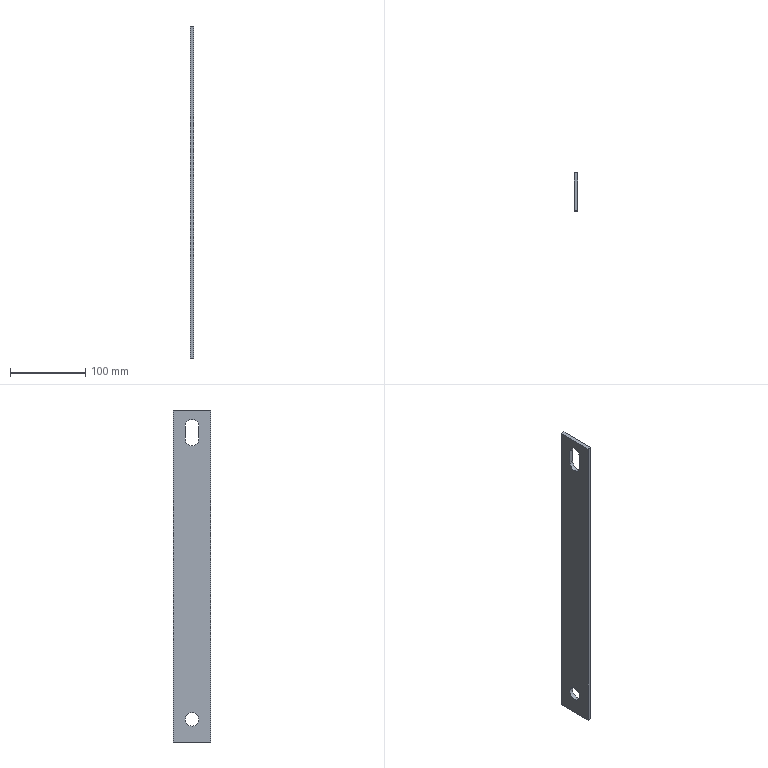Part | NX | features solid 2 | 1 solid | 11 faces | box 5 x 50 x 440 mm | volume 105925 mm3 | plane 8 | cylinder 3 | commonest cylinder face diameters 18 x3
STEP:
#1=CARTESIAN_POINT('',(1245.,-469.,203.5));
#2=VERTEX_POINT('',#1);
#3=CARTESIAN_POINT('',(1250.,-469.,203.5));
#4=VERTEX_POINT('',#3);
#5=CARTESIAN_POINT('',(1247.5,-469.,203.5));
#6=DIRECTION('',(1.,0.,0.));
#7=VECTOR('',#6,1000.);
#8=LINE('',#5,#7);
#9=EDGE_CURVE('',#2,#4,#8,.T.);
#10=ORIENTED_EDGE('',*,*,#9,.F.);
#11=CARTESIAN_POINT('',(1245.,-451.,203.5));
#12=VERTEX_POINT('',#11);
#13=CARTESIAN_POINT('',(1245.,-460.,203.5));
#14=DIRECTION('',(-1.,0.,0.));
#15=DIRECTION('',(0.,0.,1.));
#16=AXIS2_PLACEMENT_3D('',#13,#14,#15);
#17=CIRCLE('',#16,9.);
#18=EDGE_CURVE('',#2,#12,#17,.T.);
#19=ORIENTED_EDGE('',*,*,#18,.T.);
#20=CARTESIAN_POINT('',(1250.,-451.,203.5));
#21=VERTEX_POINT('',#20);
#22=CARTESIAN_POINT('',(1247.5,-451.,203.5));
#23=DIRECTION('',(-1.,0.,0.));
#24=VECTOR('',#23,1000.);
#25=LINE('',#22,#24);
#26=EDGE_CURVE('',#21,#12,#25,.T.);
#27=ORIENTED_EDGE('',*,*,#26,.F.);
#28=CARTESIAN_POINT('',(1250.,-460.,203.5));
#29=DIRECTION('',(1.,0.,0.));
#30=DIRECTION('',(0.,0.,-1.));
#31=AXIS2_PLACEMENT_3D('',#28,#29,#30);
#32=CIRCLE('',#31,9.);
#33=EDGE_CURVE('',#21,#4,#32,.T.);
#34=ORIENTED_EDGE('',*,*,#33,.T.);
#35=EDGE_LOOP('',(#10,#19,#27,#34));
#36=FACE_BOUND('',#35,.T.);
#37=CARTESIAN_POINT('',(1245.,-460.,203.5));
#38=DIRECTION('',(1.,0.,0.));
#39=DIRECTION('',(0.,0.,1.));
#40=AXIS2_PLACEMENT_3D('',#37,#38,#39);
#41=CYLINDRICAL_SURFACE('',#40,9.);
#42=ADVANCED_FACE('',(#36),#41,.F.);
#43=CARTESIAN_POINT('',(1245.,-485.,225.));
#44=VERTEX_POINT('',#43);
#45=CARTESIAN_POINT('',(1250.,-485.,225.));
#46=VERTEX_POINT('',#45);
#47=CARTESIAN_POINT('',(1247.5,-485.,225.));
#48=DIRECTION('',(1.,0.,0.));
#49=VECTOR('',#48,1000.);
#50=LINE('',#47,#49);
#51=EDGE_CURVE('',#44,#46,#50,.T.);
#52=ORIENTED_EDGE('',*,*,#51,.T.);
#53=CARTESIAN_POINT('',(1250.,-435.,225.));
#54=VERTEX_POINT('',#53);
#55=CARTESIAN_POINT('',(1250.,-460.,225.));
#56=DIRECTION('',(0.,1.,0.));
#57=VECTOR('',#56,1000.);
#58=LINE('',#55,#57);
#59=EDGE_CURVE('',#46,#54,#58,.T.);
#60=ORIENTED_EDGE('',*,*,#59,.T.);
#61=CARTESIAN_POINT('',(1245.,-435.,225.));
#62=VERTEX_POINT('',#61);
#63=CARTESIAN_POINT('',(1247.5,-435.,225.));
#64=DIRECTION('',(-1.,0.,0.));
#65=VECTOR('',#64,1000.);
#66=LINE('',#63,#65);
#67=EDGE_CURVE('',#54,#62,#66,.T.);
#68=ORIENTED_EDGE('',*,*,#67,.T.);
#69=CARTESIAN_POINT('',(1245.,-460.,225.));
#70=DIRECTION('',(0.,-1.,0.));
#71=VECTOR('',#70,1000.);
#72=LINE('',#69,#71);
#73=EDGE_CURVE('',#62,#44,#72,.T.);
#74=ORIENTED_EDGE('',*,*,#73,.T.);
#75=EDGE_LOOP('',(#52,#60,#68,#74));
#76=FACE_BOUND('',#75,.T.);
#77=CARTESIAN_POINT('',(1247.5,-460.,225.));
#78=DIRECTION('',(0.,0.,1.));
#79=DIRECTION('',(-1.,0.,0.));
#80=AXIS2_PLACEMENT_3D('',#77,#78,#79);
#81=PLANE('',#80);
#82=ADVANCED_FACE('',(#76),#81,.T.);
#83=CARTESIAN_POINT('',(1245.,-485.,-215.));
#84=VERTEX_POINT('',#83);
#85=CARTESIAN_POINT('',(1245.,-485.,-215.));
#86=DIRECTION('',(0.,0.,1.));
#87=VECTOR('',#86,1000.);
#88=LINE('',#85,#87);
#89=EDGE_CURVE('',#84,#44,#88,.T.);
#90=ORIENTED_EDGE('',*,*,#89,.F.);
#91=CARTESIAN_POINT('',(1250.,-485.,-215.));
#92=VERTEX_POINT('',#91);
#93=CARTESIAN_POINT('',(1247.5,-485.,-215.));
#94=DIRECTION('',(-1.,0.,0.));
#95=VECTOR('',#94,1000.);
#96=LINE('',#93,#95);
#97=EDGE_CURVE('',#92,#84,#96,.T.);
#98=ORIENTED_EDGE('',*,*,#97,.F.);
#99=CARTESIAN_POINT('',(1250.,-485.,-215.));
#100=DIRECTION('',(0.,0.,1.));
#101=VECTOR('',#100,1000.);
#102=LINE('',#99,#101);
#103=EDGE_CURVE('',#92,#46,#102,.T.);
#104=ORIENTED_EDGE('',*,*,#103,.T.);
#105=ORIENTED_EDGE('',*,*,#51,.F.);
#106=EDGE_LOOP('',(#90,#98,#104,#105));
#107=FACE_BOUND('',#106,.T.);
#108=CARTESIAN_POINT('',(1247.5,-485.,-215.));
#109=DIRECTION('',(0.,-1.,0.));
#110=DIRECTION('',(0.,0.,-1.));
#111=AXIS2_PLACEMENT_3D('',#108,#109,#110);
#112=PLANE('',#111);
#113=ADVANCED_FACE('',(#107),#112,.T.);
#114=CARTESIAN_POINT('',(1250.,-460.,-194.));
#115=VERTEX_POINT('',#114);
#116=CARTESIAN_POINT('',(1250.,-460.,-185.));
#117=DIRECTION('',(1.,0.,0.));
#118=DIRECTION('',(0.,0.,-1.));
#119=AXIS2_PLACEMENT_3D('',#116,#117,#118);
#120=CIRCLE('',#119,9.);
#121=EDGE_CURVE('',#115,#115,#120,.T.);
#122=ORIENTED_EDGE('',*,*,#121,.F.);
#123=EDGE_LOOP('',(#122));
#124=FACE_BOUND('',#123,.T.);
#125=CARTESIAN_POINT('',(1250.,-469.,186.5));
#126=VERTEX_POINT('',#125);
#127=CARTESIAN_POINT('',(1250.,-469.,186.5));
#128=DIRECTION('',(0.,0.,1.));
#129=VECTOR('',#128,1000.);
#130=LINE('',#127,#129);
#131=EDGE_CURVE('',#126,#4,#130,.T.);
#132=ORIENTED_EDGE('',*,*,#131,.T.);
#133=ORIENTED_EDGE('',*,*,#33,.F.);
#134=CARTESIAN_POINT('',(1250.,-451.,186.5));
#135=VERTEX_POINT('',#134);
#136=CARTESIAN_POINT('',(1250.,-451.,186.5));
#137=DIRECTION('',(0.,0.,1.));
#138=VECTOR('',#137,1000.);
#139=LINE('',#136,#138);
#140=EDGE_CURVE('',#135,#21,#139,.T.);
#141=ORIENTED_EDGE('',*,*,#140,.F.);
#142=CARTESIAN_POINT('',(1250.,-460.,186.5));
#143=DIRECTION('',(1.,0.,0.));
#144=DIRECTION('',(0.,0.,-1.));
#145=AXIS2_PLACEMENT_3D('',#142,#143,#144);
#146=CIRCLE('',#145,9.);
#147=EDGE_CURVE('',#126,#135,#146,.T.);
#148=ORIENTED_EDGE('',*,*,#147,.F.);
#149=EDGE_LOOP('',(#132,#133,#141,#148));
#150=FACE_BOUND('',#149,.T.);
#151=ORIENTED_EDGE('',*,*,#103,.F.);
#152=CARTESIAN_POINT('',(1250.,-435.,-215.));
#153=VERTEX_POINT('',#152);
#154=CARTESIAN_POINT('',(1250.,-460.,-215.));
#155=DIRECTION('',(0.,-1.,0.));
#156=VECTOR('',#155,1000.);
#157=LINE('',#154,#156);
#158=EDGE_CURVE('',#153,#92,#157,.T.);
#159=ORIENTED_EDGE('',*,*,#158,.F.);
#160=CARTESIAN_POINT('',(1250.,-435.,-215.));
#161=DIRECTION('',(0.,0.,1.));
#162=VECTOR('',#161,1000.);
#163=LINE('',#160,#162);
#164=EDGE_CURVE('',#153,#54,#163,.T.);
#165=ORIENTED_EDGE('',*,*,#164,.T.);
#166=ORIENTED_EDGE('',*,*,#59,.F.);
#167=EDGE_LOOP('',(#151,#159,#165,#166));
#168=FACE_BOUND('',#167,.T.);
#169=CARTESIAN_POINT('',(1250.,-460.,-215.));
#170=DIRECTION('',(1.,0.,0.));
#171=DIRECTION('',(0.,0.,1.));
#172=AXIS2_PLACEMENT_3D('',#169,#170,#171);
#173=PLANE('',#172);
#174=ADVANCED_FACE('',(#124,#150,#168),#173,.T.);
#175=ORIENTED_EDGE('',*,*,#164,.F.);
#176=CARTESIAN_POINT('',(1245.,-435.,-215.));
#177=VERTEX_POINT('',#176);
#178=CARTESIAN_POINT('',(1247.5,-435.,-215.));
#179=DIRECTION('',(1.,0.,0.));
#180=VECTOR('',#179,1000.);
#181=LINE('',#178,#180);
#182=EDGE_CURVE('',#177,#153,#181,.T.);
#183=ORIENTED_EDGE('',*,*,#182,.F.);
#184=CARTESIAN_POINT('',(1245.,-435.,-215.));
#185=DIRECTION('',(0.,0.,1.));
#186=VECTOR('',#185,1000.);
#187=LINE('',#184,#186);
#188=EDGE_CURVE('',#177,#62,#187,.T.);
#189=ORIENTED_EDGE('',*,*,#188,.T.);
#190=ORIENTED_EDGE('',*,*,#67,.F.);
#191=EDGE_LOOP('',(#175,#183,#189,#190));
#192=FACE_BOUND('',#191,.T.);
#193=CARTESIAN_POINT('',(1247.5,-435.,-215.));
#194=DIRECTION('',(0.,1.,0.));
#195=DIRECTION('',(0.,0.,1.));
#196=AXIS2_PLACEMENT_3D('',#193,#194,#195);
#197=PLANE('',#196);
#198=ADVANCED_FACE('',(#192),#197,.T.);
#199=CARTESIAN_POINT('',(1245.,-460.,-215.));
#200=DIRECTION('',(0.,1.,0.));
#201=VECTOR('',#200,1000.);
#202=LINE('',#199,#201);
#203=EDGE_CURVE('',#84,#177,#202,.T.);
#204=ORIENTED_EDGE('',*,*,#203,.T.);
#205=ORIENTED_EDGE('',*,*,#182,.T.);
#206=ORIENTED_EDGE('',*,*,#158,.T.);
#207=ORIENTED_EDGE('',*,*,#97,.T.);
#208=EDGE_LOOP('',(#204,#205,#206,#207));
#209=FACE_BOUND('',#208,.T.);
#210=CARTESIAN_POINT('',(1247.5,-460.,-215.));
#211=DIRECTION('',(0.,0.,-1.));
#212=DIRECTION('',(1.,0.,0.));
#213=AXIS2_PLACEMENT_3D('',#210,#211,#212);
#214=PLANE('',#213);
#215=ADVANCED_FACE('',(#209),#214,.T.);
#216=CARTESIAN_POINT('',(1245.,-460.,-176.));
#217=VERTEX_POINT('',#216);
#218=CARTESIAN_POINT('',(1245.,-460.,-185.));
#219=DIRECTION('',(-1.,0.,0.));
#220=DIRECTION('',(0.,0.,1.));
#221=AXIS2_PLACEMENT_3D('',#218,#219,#220);
#222=CIRCLE('',#221,9.);
#223=EDGE_CURVE('',#217,#217,#222,.T.);
#224=ORIENTED_EDGE('',*,*,#223,.F.);
#225=EDGE_LOOP('',(#224));
#226=FACE_BOUND('',#225,.T.);
#227=CARTESIAN_POINT('',(1245.,-469.,186.5));
#228=VERTEX_POINT('',#227);
#229=CARTESIAN_POINT('',(1245.,-469.,186.5));
#230=DIRECTION('',(0.,0.,1.));
#231=VECTOR('',#230,1000.);
#232=LINE('',#229,#231);
#233=EDGE_CURVE('',#228,#2,#232,.T.);
#234=ORIENTED_EDGE('',*,*,#233,.F.);
#235=CARTESIAN_POINT('',(1245.,-451.,186.5));
#236=VERTEX_POINT('',#235);
#237=CARTESIAN_POINT('',(1245.,-460.,186.5));
#238=DIRECTION('',(-1.,0.,0.));
#239=DIRECTION('',(0.,0.,1.));
#240=AXIS2_PLACEMENT_3D('',#237,#238,#239);
#241=CIRCLE('',#240,9.);
#242=EDGE_CURVE('',#236,#228,#241,.T.);
#243=ORIENTED_EDGE('',*,*,#242,.F.);
#244=CARTESIAN_POINT('',(1245.,-451.,186.5));
#245=DIRECTION('',(0.,0.,1.));
#246=VECTOR('',#245,1000.);
#247=LINE('',#244,#246);
#248=EDGE_CURVE('',#236,#12,#247,.T.);
#249=ORIENTED_EDGE('',*,*,#248,.T.);
#250=ORIENTED_EDGE('',*,*,#18,.F.);
#251=EDGE_LOOP('',(#234,#243,#249,#250));
#252=FACE_BOUND('',#251,.T.);
#253=ORIENTED_EDGE('',*,*,#203,.F.);
#254=ORIENTED_EDGE('',*,*,#89,.T.);
#255=ORIENTED_EDGE('',*,*,#73,.F.);
#256=ORIENTED_EDGE('',*,*,#188,.F.);
#257=EDGE_LOOP('',(#253,#254,#255,#256));
#258=FACE_BOUND('',#257,.T.);
#259=CARTESIAN_POINT('',(1245.,-460.,-215.));
#260=DIRECTION('',(-1.,0.,0.));
#261=DIRECTION('',(0.,0.,-1.));
#262=AXIS2_PLACEMENT_3D('',#259,#260,#261);
#263=PLANE('',#262);
#264=ADVANCED_FACE('',(#226,#252,#258),#263,.T.);
#265=ORIENTED_EDGE('',*,*,#147,.T.);
#266=CARTESIAN_POINT('',(1247.5,-451.,186.5));
#267=DIRECTION('',(1.,0.,0.));
#268=VECTOR('',#267,1000.);
#269=LINE('',#266,#268);
#270=EDGE_CURVE('',#236,#135,#269,.T.);
#271=ORIENTED_EDGE('',*,*,#270,.F.);
#272=ORIENTED_EDGE('',*,*,#242,.T.);
#273=CARTESIAN_POINT('',(1247.5,-469.,186.5));
#274=DIRECTION('',(-1.,0.,0.));
#275=VECTOR('',#274,1000.);
#276=LINE('',#273,#275);
#277=EDGE_CURVE('',#126,#228,#276,.T.);
#278=ORIENTED_EDGE('',*,*,#277,.F.);
#279=EDGE_LOOP('',(#265,#271,#272,#278));
#280=FACE_BOUND('',#279,.T.);
#281=CARTESIAN_POINT('',(1245.,-460.,186.5));
#282=DIRECTION('',(1.,0.,0.));
#283=DIRECTION('',(0.,0.,1.));
#284=AXIS2_PLACEMENT_3D('',#281,#282,#283);
#285=CYLINDRICAL_SURFACE('',#284,9.);
#286=ADVANCED_FACE('',(#280),#285,.F.);
#287=ORIENTED_EDGE('',*,*,#140,.T.);
#288=ORIENTED_EDGE('',*,*,#26,.T.);
#289=ORIENTED_EDGE('',*,*,#248,.F.);
#290=ORIENTED_EDGE('',*,*,#270,.T.);
#291=EDGE_LOOP('',(#287,#288,#289,#290));
#292=FACE_BOUND('',#291,.T.);
#293=CARTESIAN_POINT('',(1247.5,-451.,186.5));
#294=DIRECTION('',(0.,1.,0.));
#295=DIRECTION('',(0.,0.,1.));
#296=AXIS2_PLACEMENT_3D('',#293,#294,#295);
#297=PLANE('',#296);
#298=ADVANCED_FACE('',(#292),#297,.F.);
#299=ORIENTED_EDGE('',*,*,#233,.T.);
#300=ORIENTED_EDGE('',*,*,#9,.T.);
#301=ORIENTED_EDGE('',*,*,#131,.F.);
#302=ORIENTED_EDGE('',*,*,#277,.T.);
#303=EDGE_LOOP('',(#299,#300,#301,#302));
#304=FACE_BOUND('',#303,.T.);
#305=CARTESIAN_POINT('',(1247.5,-469.,186.5));
#306=DIRECTION('',(0.,-1.,0.));
#307=DIRECTION('',(0.,0.,-1.));
#308=AXIS2_PLACEMENT_3D('',#305,#306,#307);
#309=PLANE('',#308);
#310=ADVANCED_FACE('',(#304),#309,.F.);
#311=ORIENTED_EDGE('',*,*,#121,.T.);
#312=EDGE_LOOP('',(#311));
#313=FACE_BOUND('',#312,.T.);
#314=ORIENTED_EDGE('',*,*,#223,.T.);
#315=EDGE_LOOP('',(#314));
#316=FACE_BOUND('',#315,.T.);
#317=CARTESIAN_POINT('',(1245.,-460.,-185.));
#318=DIRECTION('',(1.,0.,0.));
#319=DIRECTION('',(0.,0.,1.));
#320=AXIS2_PLACEMENT_3D('',#317,#318,#319);
#321=CYLINDRICAL_SURFACE('',#320,9.);
#322=ADVANCED_FACE('',(#313,#316),#321,.F.);
#323=CLOSED_SHELL('',(#42,#82,#113,#174,#198,#215,#264,#286,#298,#310,#322));
#324=MANIFOLD_SOLID_BREP('',#323);
#325=(LENGTH_UNIT()NAMED_UNIT(*)SI_UNIT(.MILLI.,.METRE.));
#326=UNCERTAINTY_MEASURE_WITH_UNIT(LENGTH_MEASURE(0.00001),#325,'','');
#327=(NAMED_UNIT(*)PLANE_ANGLE_UNIT()SI_UNIT($,.RADIAN.));
#328=(NAMED_UNIT(*)SI_UNIT($,.STERADIAN.)SOLID_ANGLE_UNIT());
#329=(GEOMETRIC_REPRESENTATION_CONTEXT(3)GLOBAL_UNCERTAINTY_ASSIGNED_CONTEXT((#326))GLOBAL_UNIT_ASSIGNED_CONTEXT((#325,#327,#328))REPRESENTATION_CONTEXT('',''));
#330=ADVANCED_BREP_SHAPE_REPRESENTATION('',(#324),#329);